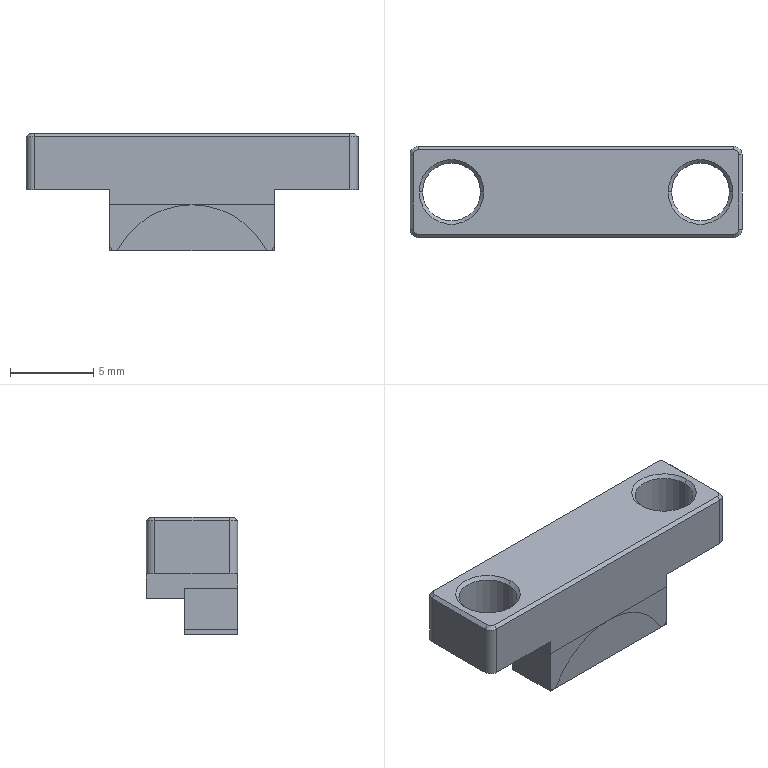Part | 2 solids | 42 faces | box 20 x 5.5 x 7.057 mm | volume 487.21 mm3 | plane 23 | cylinder 11 | cone 8 | commonest cylinder face diameters 1 x4 3.5 x4 0.6 x2 10 x1
STEP:
#1=CARTESIAN_POINT('',(4.95,-2.75,-4.3));
#2=VERTEX_POINT('',#1);
#3=CARTESIAN_POINT('',(-4.95,-2.75,-4.3));
#4=VERTEX_POINT('',#3);
#5=CARTESIAN_POINT('',(0.,-2.75,-4.3));
#6=DIRECTION('',(-1.,0.,0.));
#7=VECTOR('',#6,1000.);
#8=LINE('',#5,#7);
#9=EDGE_CURVE('',#2,#4,#8,.T.);
#10=ORIENTED_EDGE('',*,*,#9,.F.);
#11=CARTESIAN_POINT('',(4.95,0.45,-4.3));
#12=VERTEX_POINT('',#11);
#13=CARTESIAN_POINT('',(4.95,-1.15,-4.3));
#14=DIRECTION('',(0.,-1.,0.));
#15=VECTOR('',#14,1000.);
#16=LINE('',#13,#15);
#17=EDGE_CURVE('',#12,#2,#16,.T.);
#18=ORIENTED_EDGE('',*,*,#17,.F.);
#19=CARTESIAN_POINT('',(-4.95,0.45,-4.3));
#20=VERTEX_POINT('',#19);
#21=CARTESIAN_POINT('',(0.,0.45,-4.3));
#22=DIRECTION('',(1.,0.,0.));
#23=VECTOR('',#22,1000.);
#24=LINE('',#21,#23);
#25=EDGE_CURVE('',#20,#12,#24,.T.);
#26=ORIENTED_EDGE('',*,*,#25,.F.);
#27=CARTESIAN_POINT('',(-4.95,-1.15,-4.3));
#28=DIRECTION('',(0.,1.,0.));
#29=VECTOR('',#28,1000.);
#30=LINE('',#27,#29);
#31=EDGE_CURVE('',#4,#20,#30,.T.);
#32=ORIENTED_EDGE('',*,*,#31,.F.);
#33=EDGE_LOOP('',(#10,#18,#26,#32));
#34=FACE_BOUND('',#33,.T.);
#35=CARTESIAN_POINT('',(0.,-1.15,-4.3));
#36=DIRECTION('',(0.,0.,1.));
#37=DIRECTION('',(1.,0.,0.));
#38=AXIS2_PLACEMENT_3D('',#35,#36,#37);
#39=PLANE('',#38);
#40=ADVANCED_FACE('',(#34),#39,.T.);
#41=CARTESIAN_POINT('',(4.95,-2.75,-7.057));
#42=VERTEX_POINT('',#41);
#43=CARTESIAN_POINT('',(4.95,-2.75,-7.057));
#44=DIRECTION('',(0.,0.,1.));
#45=VECTOR('',#44,1000.);
#46=LINE('',#43,#45);
#47=EDGE_CURVE('',#42,#2,#46,.T.);
#48=ORIENTED_EDGE('',*,*,#47,.T.);
#49=ORIENTED_EDGE('',*,*,#9,.T.);
#50=CARTESIAN_POINT('',(-4.95,-2.75,-7.057));
#51=VERTEX_POINT('',#50);
#52=CARTESIAN_POINT('',(-4.95,-2.75,-7.057));
#53=DIRECTION('',(0.,0.,1.));
#54=VECTOR('',#53,1000.);
#55=LINE('',#52,#54);
#56=EDGE_CURVE('',#51,#4,#55,.T.);
#57=ORIENTED_EDGE('',*,*,#56,.F.);
#58=CARTESIAN_POINT('',(0.,-2.75,-7.057));
#59=DIRECTION('',(1.,0.,0.));
#60=VECTOR('',#59,1000.);
#61=LINE('',#58,#60);
#62=EDGE_CURVE('',#51,#42,#61,.T.);
#63=ORIENTED_EDGE('',*,*,#62,.T.);
#64=EDGE_LOOP('',(#48,#49,#57,#63));
#65=FACE_BOUND('',#64,.T.);
#66=CARTESIAN_POINT('',(0.,-2.75,-7.057));
#67=DIRECTION('',(0.,-1.,0.));
#68=DIRECTION('',(0.,0.,-1.));
#69=AXIS2_PLACEMENT_3D('',#66,#67,#68);
#70=PLANE('',#69);
#71=ADVANCED_FACE('',(#65),#70,.T.);
#72=ORIENTED_EDGE('',*,*,#56,.T.);
#73=ORIENTED_EDGE('',*,*,#31,.T.);
#74=CARTESIAN_POINT('',(-4.95,0.45,-7.057));
#75=VERTEX_POINT('',#74);
#76=CARTESIAN_POINT('',(-4.95,0.45,-7.057));
#77=DIRECTION('',(0.,0.,1.));
#78=VECTOR('',#77,1000.);
#79=LINE('',#76,#78);
#80=EDGE_CURVE('',#75,#20,#79,.T.);
#81=ORIENTED_EDGE('',*,*,#80,.F.);
#82=CARTESIAN_POINT('',(-4.95,-1.15,-7.057));
#83=DIRECTION('',(0.,-1.,0.));
#84=VECTOR('',#83,1000.);
#85=LINE('',#82,#84);
#86=EDGE_CURVE('',#75,#51,#85,.T.);
#87=ORIENTED_EDGE('',*,*,#86,.T.);
#88=EDGE_LOOP('',(#72,#73,#81,#87));
#89=FACE_BOUND('',#88,.T.);
#90=CARTESIAN_POINT('',(-4.95,-1.15,-7.057));
#91=DIRECTION('',(-1.,0.,0.));
#92=DIRECTION('',(0.,0.,1.));
#93=AXIS2_PLACEMENT_3D('',#90,#91,#92);
#94=PLANE('',#93);
#95=ADVANCED_FACE('',(#89),#94,.T.);
#96=ORIENTED_EDGE('',*,*,#80,.T.);
#97=ORIENTED_EDGE('',*,*,#25,.T.);
#98=CARTESIAN_POINT('',(4.95,0.45,-7.057));
#99=VERTEX_POINT('',#98);
#100=CARTESIAN_POINT('',(4.95,0.45,-7.057));
#101=DIRECTION('',(0.,0.,1.));
#102=VECTOR('',#101,1000.);
#103=LINE('',#100,#102);
#104=EDGE_CURVE('',#99,#12,#103,.T.);
#105=ORIENTED_EDGE('',*,*,#104,.F.);
#106=CARTESIAN_POINT('',(0.,0.45,-7.057));
#107=DIRECTION('',(-1.,0.,0.));
#108=VECTOR('',#107,1000.);
#109=LINE('',#106,#108);
#110=EDGE_CURVE('',#99,#75,#109,.T.);
#111=ORIENTED_EDGE('',*,*,#110,.T.);
#112=EDGE_LOOP('',(#96,#97,#105,#111));
#113=FACE_BOUND('',#112,.T.);
#114=CARTESIAN_POINT('',(0.,0.45,-7.057));
#115=DIRECTION('',(0.,1.,0.));
#116=DIRECTION('',(0.,0.,1.));
#117=AXIS2_PLACEMENT_3D('',#114,#115,#116);
#118=PLANE('',#117);
#119=ADVANCED_FACE('',(#113),#118,.T.);
#120=CARTESIAN_POINT('',(4.95,-1.15,-7.057));
#121=DIRECTION('',(0.,1.,0.));
#122=VECTOR('',#121,1000.);
#123=LINE('',#120,#122);
#124=EDGE_CURVE('',#42,#99,#123,.T.);
#125=ORIENTED_EDGE('',*,*,#124,.F.);
#126=ORIENTED_EDGE('',*,*,#62,.F.);
#127=ORIENTED_EDGE('',*,*,#86,.F.);
#128=ORIENTED_EDGE('',*,*,#110,.F.);
#129=EDGE_LOOP('',(#125,#126,#127,#128));
#130=FACE_BOUND('',#129,.T.);
#131=CARTESIAN_POINT('',(0.,-1.15,-7.057));
#132=DIRECTION('',(0.,0.,-1.));
#133=DIRECTION('',(-1.,0.,0.));
#134=AXIS2_PLACEMENT_3D('',#131,#132,#133);
#135=PLANE('',#134);
#136=ADVANCED_FACE('',(#130),#135,.T.);
#137=ORIENTED_EDGE('',*,*,#124,.T.);
#138=ORIENTED_EDGE('',*,*,#104,.T.);
#139=ORIENTED_EDGE('',*,*,#17,.T.);
#140=ORIENTED_EDGE('',*,*,#47,.F.);
#141=EDGE_LOOP('',(#137,#138,#139,#140));
#142=FACE_BOUND('',#141,.T.);
#143=CARTESIAN_POINT('',(4.95,-1.15,-7.057));
#144=DIRECTION('',(1.,0.,0.));
#145=DIRECTION('',(0.,0.,-1.));
#146=AXIS2_PLACEMENT_3D('',#143,#144,#145);
#147=PLANE('',#146);
#148=ADVANCED_FACE('',(#142),#147,.T.);
#149=CLOSED_SHELL('',(#40,#71,#95,#119,#136,#148));
#150=MANIFOLD_SOLID_BREP('',#149);
#151=CARTESIAN_POINT('',(9.5,2.75,-0.2));
#152=VERTEX_POINT('',#151);
#153=CARTESIAN_POINT('',(9.5,2.75,-3.4));
#154=VERTEX_POINT('',#153);
#155=CARTESIAN_POINT('',(9.5,2.75,-0.2));
#156=DIRECTION('',(-0.000000324,0.000000043,-1.));
#157=VECTOR('',#156,1000.);
#158=LINE('',#155,#157);
#159=EDGE_CURVE('',#152,#154,#158,.T.);
#160=ORIENTED_EDGE('',*,*,#159,.T.);
#161=CARTESIAN_POINT('',(4.95,2.75,-3.4));
#162=VERTEX_POINT('',#161);
#163=CARTESIAN_POINT('',(4.95,2.75,-3.4));
#164=DIRECTION('',(1.,0.,0.));
#165=VECTOR('',#164,1000.);
#166=LINE('',#163,#165);
#167=EDGE_CURVE('',#162,#154,#166,.T.);
#168=ORIENTED_EDGE('',*,*,#167,.F.);
#169=CARTESIAN_POINT('',(4.95,2.75,-4.9));
#170=VERTEX_POINT('',#169);
#171=CARTESIAN_POINT('',(4.95,2.75,-3.4));
#172=DIRECTION('',(0.,0.,-1.));
#173=VECTOR('',#172,1000.);
#174=LINE('',#171,#173);
#175=EDGE_CURVE('',#162,#170,#174,.T.);
#176=ORIENTED_EDGE('',*,*,#175,.T.);
#177=CARTESIAN_POINT('',(-4.95,2.75,-4.9));
#178=VERTEX_POINT('',#177);
#179=CARTESIAN_POINT('',(4.95,2.75,-4.9));
#180=DIRECTION('',(-1.,0.,0.));
#181=VECTOR('',#180,1000.);
#182=LINE('',#179,#181);
#183=EDGE_CURVE('',#170,#178,#182,.T.);
#184=ORIENTED_EDGE('',*,*,#183,.T.);
#185=CARTESIAN_POINT('',(-4.95,2.75,-3.4));
#186=VERTEX_POINT('',#185);
#187=CARTESIAN_POINT('',(-4.95,2.75,-4.9));
#188=DIRECTION('',(0.,0.,1.));
#189=VECTOR('',#188,1000.);
#190=LINE('',#187,#189);
#191=EDGE_CURVE('',#178,#186,#190,.T.);
#192=ORIENTED_EDGE('',*,*,#191,.T.);
#193=CARTESIAN_POINT('',(-9.5,2.75,-3.4));
#194=VERTEX_POINT('',#193);
#195=CARTESIAN_POINT('',(-9.5,2.75,-3.4));
#196=DIRECTION('',(1.,0.,0.));
#197=VECTOR('',#196,1000.);
#198=LINE('',#195,#197);
#199=EDGE_CURVE('',#194,#186,#198,.T.);
#200=ORIENTED_EDGE('',*,*,#199,.F.);
#201=CARTESIAN_POINT('',(-9.5,2.75,-0.2));
#202=VERTEX_POINT('',#201);
#203=CARTESIAN_POINT('',(-9.5,2.75,-3.4));
#204=DIRECTION('',(-0.000000324,-0.000000043,1.));
#205=VECTOR('',#204,1000.);
#206=LINE('',#203,#205);
#207=EDGE_CURVE('',#194,#202,#206,.T.);
#208=ORIENTED_EDGE('',*,*,#207,.T.);
#209=CARTESIAN_POINT('',(-9.5,2.75,-0.2));
#210=DIRECTION('',(1.,0.,0.));
#211=VECTOR('',#210,1000.);
#212=LINE('',#209,#211);
#213=EDGE_CURVE('',#202,#152,#212,.T.);
#214=ORIENTED_EDGE('',*,*,#213,.T.);
#215=EDGE_LOOP('',(#160,#168,#176,#184,#192,#200,#208,#214));
#216=FACE_BOUND('',#215,.T.);
#217=CARTESIAN_POINT('',(0.,2.75,-8.9));
#218=DIRECTION('',(0.,-1.,0.));
#219=DIRECTION('',(-1.,0.,0.));
#220=AXIS2_PLACEMENT_3D('',#217,#218,#219);
#221=PLANE('',#220);
#222=ADVANCED_FACE('',(#216),#221,.F.);
#223=CARTESIAN_POINT('',(-9.5,2.55,0.));
#224=VERTEX_POINT('',#223);
#225=CARTESIAN_POINT('',(-9.5,2.75,-0.2));
#226=DIRECTION('',(0.000000734,-0.7071,0.7071));
#227=VECTOR('',#226,1000.);
#228=LINE('',#225,#227);
#229=EDGE_CURVE('',#202,#224,#228,.T.);
#230=ORIENTED_EDGE('',*,*,#229,.T.);
#231=CARTESIAN_POINT('',(9.5,2.55,0.));
#232=VERTEX_POINT('',#231);
#233=CARTESIAN_POINT('',(-9.5,2.55,0.000000111));
#234=DIRECTION('',(1.,0.,0.));
#235=VECTOR('',#234,1000.);
#236=LINE('',#233,#235);
#237=EDGE_CURVE('',#224,#232,#236,.T.);
#238=ORIENTED_EDGE('',*,*,#237,.T.);
#239=CARTESIAN_POINT('',(9.5,2.75,-0.2));
#240=DIRECTION('',(-0.000000734,-0.7071,0.7071));
#241=VECTOR('',#240,1000.);
#242=LINE('',#239,#241);
#243=EDGE_CURVE('',#152,#232,#242,.T.);
#244=ORIENTED_EDGE('',*,*,#243,.F.);
#245=ORIENTED_EDGE('',*,*,#213,.F.);
#246=EDGE_LOOP('',(#230,#238,#244,#245));
#247=FACE_BOUND('',#246,.T.);
#248=CARTESIAN_POINT('',(0.,2.65,-0.1));
#249=DIRECTION('',(0.,0.7071,0.7071));
#250=DIRECTION('',(0.,0.7071,-0.7071));
#251=AXIS2_PLACEMENT_3D('',#248,#249,#250);
#252=PLANE('',#251);
#253=ADVANCED_FACE('',(#247),#252,.T.);
#254=ORIENTED_EDGE('',*,*,#243,.T.);
#255=CARTESIAN_POINT('',(9.8,2.25,0.));
#256=VERTEX_POINT('',#255);
#257=CARTESIAN_POINT('',(9.5,2.25,0.));
#258=DIRECTION('',(0.,0.,-1.));
#259=DIRECTION('',(0.,1.,0.));
#260=AXIS2_PLACEMENT_3D('',#257,#258,#259);
#261=CIRCLE('',#260,0.3);
#262=EDGE_CURVE('',#232,#256,#261,.T.);
#263=ORIENTED_EDGE('',*,*,#262,.T.);
#264=CARTESIAN_POINT('',(10.,2.25,-0.2));
#265=VERTEX_POINT('',#264);
#266=CARTESIAN_POINT('',(10.,2.25,-0.2));
#267=DIRECTION('',(-0.7071,-0.000000602,0.7071));
#268=VECTOR('',#267,1000.);
#269=LINE('',#266,#268);
#270=EDGE_CURVE('',#265,#256,#269,.T.);
#271=ORIENTED_EDGE('',*,*,#270,.F.);
#272=CARTESIAN_POINT('',(9.5,2.25,-0.2));
#273=DIRECTION('',(0.,0.,-1.));
#274=DIRECTION('',(0.,1.,0.));
#275=AXIS2_PLACEMENT_3D('',#272,#273,#274);
#276=CIRCLE('',#275,0.5);
#277=EDGE_CURVE('',#152,#265,#276,.T.);
#278=ORIENTED_EDGE('',*,*,#277,.F.);
#279=EDGE_LOOP('',(#254,#263,#271,#278));
#280=FACE_BOUND('',#279,.T.);
#281=CARTESIAN_POINT('',(9.5,2.25,-0.1));
#282=DIRECTION('',(0.,0.,-1.));
#283=DIRECTION('',(1.,0.,0.));
#284=AXIS2_PLACEMENT_3D('',#281,#282,#283);
#285=CONICAL_SURFACE('',#284,0.4,0.7854);
#286=ADVANCED_FACE('',(#280),#285,.T.);
#287=CARTESIAN_POINT('',(10.,2.25,-3.4));
#288=VERTEX_POINT('',#287);
#289=CARTESIAN_POINT('',(10.,2.25,-0.2));
#290=DIRECTION('',(0.000000046,-0.000000266,-1.));
#291=VECTOR('',#290,1000.);
#292=LINE('',#289,#291);
#293=EDGE_CURVE('',#265,#288,#292,.T.);
#294=ORIENTED_EDGE('',*,*,#293,.T.);
#295=CARTESIAN_POINT('',(9.5,2.25,-3.4));
#296=DIRECTION('',(0.,0.,-1.));
#297=DIRECTION('',(0.,1.,0.));
#298=AXIS2_PLACEMENT_3D('',#295,#296,#297);
#299=CIRCLE('',#298,0.5);
#300=EDGE_CURVE('',#154,#288,#299,.T.);
#301=ORIENTED_EDGE('',*,*,#300,.F.);
#302=ORIENTED_EDGE('',*,*,#159,.F.);
#303=ORIENTED_EDGE('',*,*,#277,.T.);
#304=EDGE_LOOP('',(#294,#301,#302,#303));
#305=FACE_BOUND('',#304,.T.);
#306=CARTESIAN_POINT('',(9.5,2.25,6.388));
#307=DIRECTION('',(0.,0.,-1.));
#308=DIRECTION('',(0.,-1.,0.));
#309=AXIS2_PLACEMENT_3D('',#306,#307,#308);
#310=CYLINDRICAL_SURFACE('',#309,0.5);
#311=ADVANCED_FACE('',(#305),#310,.T.);
#312=ORIENTED_EDGE('',*,*,#300,.T.);
#313=CARTESIAN_POINT('',(10.,-2.25,-3.4));
#314=VERTEX_POINT('',#313);
#315=CARTESIAN_POINT('',(10.,2.25,-3.4));
#316=DIRECTION('',(0.,-1.,0.));
#317=VECTOR('',#316,1000.);
#318=LINE('',#315,#317);
#319=EDGE_CURVE('',#288,#314,#318,.T.);
#320=ORIENTED_EDGE('',*,*,#319,.T.);
#321=CARTESIAN_POINT('',(9.5,-2.75,-3.4));
#322=VERTEX_POINT('',#321);
#323=CARTESIAN_POINT('',(9.5,-2.25,-3.4));
#324=DIRECTION('',(0.,0.,-1.));
#325=DIRECTION('',(1.,0.,0.));
#326=AXIS2_PLACEMENT_3D('',#323,#324,#325);
#327=CIRCLE('',#326,0.5);
#328=EDGE_CURVE('',#314,#322,#327,.T.);
#329=ORIENTED_EDGE('',*,*,#328,.T.);
#330=CARTESIAN_POINT('',(4.95,-2.75,-3.4));
#331=VERTEX_POINT('',#330);
#332=CARTESIAN_POINT('',(4.95,-2.75,-3.4));
#333=DIRECTION('',(1.,0.,0.));
#334=VECTOR('',#333,1000.);
#335=LINE('',#332,#334);
#336=EDGE_CURVE('',#331,#322,#335,.T.);
#337=ORIENTED_EDGE('',*,*,#336,.F.);
#338=CARTESIAN_POINT('',(4.95,2.75,-3.4));
#339=DIRECTION('',(0.,-1.,0.));
#340=VECTOR('',#339,1000.);
#341=LINE('',#338,#340);
#342=EDGE_CURVE('',#162,#331,#341,.T.);
#343=ORIENTED_EDGE('',*,*,#342,.F.);
#344=ORIENTED_EDGE('',*,*,#167,.T.);
#345=EDGE_LOOP('',(#312,#320,#329,#337,#343,#344));
#346=FACE_BOUND('',#345,.T.);
#347=CARTESIAN_POINT('',(5.75,0.,-3.4));
#348=VERTEX_POINT('',#347);
#349=CARTESIAN_POINT('',(9.25,0.,-3.4));
#350=VERTEX_POINT('',#349);
#351=CARTESIAN_POINT('',(7.5,0.,-3.4));
#352=DIRECTION('',(0.,0.,1.));
#353=DIRECTION('',(-1.,0.,0.));
#354=AXIS2_PLACEMENT_3D('',#351,#352,#353);
#355=CIRCLE('',#354,1.75);
#356=EDGE_CURVE('',#348,#350,#355,.T.);
#357=ORIENTED_EDGE('',*,*,#356,.T.);
#358=CARTESIAN_POINT('',(7.5,0.,-3.4));
#359=DIRECTION('',(0.,0.,1.));
#360=DIRECTION('',(1.,0.,0.));
#361=AXIS2_PLACEMENT_3D('',#358,#359,#360);
#362=CIRCLE('',#361,1.75);
#363=EDGE_CURVE('',#350,#348,#362,.T.);
#364=ORIENTED_EDGE('',*,*,#363,.T.);
#365=EDGE_LOOP('',(#357,#364));
#366=FACE_BOUND('',#365,.T.);
#367=CARTESIAN_POINT('',(4.95,2.75,-3.4));
#368=DIRECTION('',(0.,0.,-1.));
#369=DIRECTION('',(-1.,0.,0.));
#370=AXIS2_PLACEMENT_3D('',#367,#368,#369);
#371=PLANE('',#370);
#372=ADVANCED_FACE('',(#346,#366),#371,.T.);
#373=CARTESIAN_POINT('',(5.75,0.,-0.2));
#374=VERTEX_POINT('',#373);
#375=CARTESIAN_POINT('',(5.75,0.000000759,-0.2));
#376=DIRECTION('',(-0.00000006,-0.000000237,-1.));
#377=VECTOR('',#376,1000.);
#378=LINE('',#375,#377);
#379=EDGE_CURVE('',#374,#348,#378,.T.);
#380=ORIENTED_EDGE('',*,*,#379,.T.);
#381=ORIENTED_EDGE('',*,*,#363,.F.);
#382=CARTESIAN_POINT('',(9.25,0.,-0.2));
#383=VERTEX_POINT('',#382);
#384=CARTESIAN_POINT('',(9.25,-0.000000759,-0.2));
#385=DIRECTION('',(0.00000006,0.000000237,-1.));
#386=VECTOR('',#385,1000.);
#387=LINE('',#384,#386);
#388=EDGE_CURVE('',#383,#350,#387,.T.);
#389=ORIENTED_EDGE('',*,*,#388,.F.);
#390=CARTESIAN_POINT('',(7.5,0.,-0.2));
#391=DIRECTION('',(0.,0.,-1.));
#392=DIRECTION('',(-1.,0.,0.));
#393=AXIS2_PLACEMENT_3D('',#390,#391,#392);
#394=CIRCLE('',#393,1.75);
#395=EDGE_CURVE('',#374,#383,#394,.T.);
#396=ORIENTED_EDGE('',*,*,#395,.F.);
#397=EDGE_LOOP('',(#380,#381,#389,#396));
#398=FACE_BOUND('',#397,.T.);
#399=CARTESIAN_POINT('',(7.5,0.,0.));
#400=DIRECTION('',(0.,0.,1.));
#401=DIRECTION('',(-1.,0.,0.));
#402=AXIS2_PLACEMENT_3D('',#399,#400,#401);
#403=CYLINDRICAL_SURFACE('',#402,1.75);
#404=ADVANCED_FACE('',(#398),#403,.F.);
#405=CARTESIAN_POINT('',(5.55,0.,0.));
#406=VERTEX_POINT('',#405);
#407=CARTESIAN_POINT('',(5.55,0.000001127,-0.000000285));
#408=DIRECTION('',(0.7071,-0.000001303,-0.7071));
#409=VECTOR('',#408,1000.);
#410=LINE('',#407,#409);
#411=EDGE_CURVE('',#406,#374,#410,.T.);
#412=ORIENTED_EDGE('',*,*,#411,.T.);
#413=ORIENTED_EDGE('',*,*,#395,.T.);
#414=CARTESIAN_POINT('',(9.45,0.,0.));
#415=VERTEX_POINT('',#414);
#416=CARTESIAN_POINT('',(9.45,-0.000001127,-0.000000285));
#417=DIRECTION('',(-0.7071,0.000001303,-0.7071));
#418=VECTOR('',#417,1000.);
#419=LINE('',#416,#418);
#420=EDGE_CURVE('',#415,#383,#419,.T.);
#421=ORIENTED_EDGE('',*,*,#420,.F.);
#422=CARTESIAN_POINT('',(7.5,0.,0.));
#423=DIRECTION('',(0.,0.,-1.));
#424=DIRECTION('',(-1.,0.,0.));
#425=AXIS2_PLACEMENT_3D('',#422,#423,#424);
#426=CIRCLE('',#425,1.95);
#427=EDGE_CURVE('',#406,#415,#426,.T.);
#428=ORIENTED_EDGE('',*,*,#427,.F.);
#429=EDGE_LOOP('',(#412,#413,#421,#428));
#430=FACE_BOUND('',#429,.T.);
#431=CARTESIAN_POINT('',(7.5,0.,-0.1));
#432=DIRECTION('',(0.,0.,1.));
#433=DIRECTION('',(1.,0.,0.));
#434=AXIS2_PLACEMENT_3D('',#431,#432,#433);
#435=CONICAL_SURFACE('',#434,1.85,0.7854);
#436=ADVANCED_FACE('',(#430),#435,.F.);
#437=ORIENTED_EDGE('',*,*,#237,.F.);
#438=CARTESIAN_POINT('',(-9.8,2.25,0.000000117));
#439=VERTEX_POINT('',#438);
#440=CARTESIAN_POINT('',(-9.5,2.25,0.));
#441=DIRECTION('',(0.,0.,-1.));
#442=DIRECTION('',(-1.,0.,0.));
#443=AXIS2_PLACEMENT_3D('',#440,#441,#442);
#444=CIRCLE('',#443,0.3);
#445=EDGE_CURVE('',#439,#224,#444,.T.);
#446=ORIENTED_EDGE('',*,*,#445,.F.);
#447=CARTESIAN_POINT('',(-9.8,-2.25,0.));
#448=VERTEX_POINT('',#447);
#449=CARTESIAN_POINT('',(-9.8,-2.25,0.000000117));
#450=DIRECTION('',(0.,1.,0.));
#451=VECTOR('',#450,1000.);
#452=LINE('',#449,#451);
#453=EDGE_CURVE('',#448,#439,#452,.T.);
#454=ORIENTED_EDGE('',*,*,#453,.F.);
#455=CARTESIAN_POINT('',(-9.5,-2.55,0.000000111));
#456=VERTEX_POINT('',#455);
#457=CARTESIAN_POINT('',(-9.5,-2.25,0.));
#458=DIRECTION('',(0.,0.,-1.));
#459=DIRECTION('',(0.,-1.,0.));
#460=AXIS2_PLACEMENT_3D('',#457,#458,#459);
#461=CIRCLE('',#460,0.3);
#462=EDGE_CURVE('',#456,#448,#461,.T.);
#463=ORIENTED_EDGE('',*,*,#462,.F.);
#464=CARTESIAN_POINT('',(9.5,-2.55,0.));
#465=VERTEX_POINT('',#464);
#466=CARTESIAN_POINT('',(9.5,-2.55,0.000000111));
#467=DIRECTION('',(-1.,0.,0.));
#468=VECTOR('',#467,1000.);
#469=LINE('',#466,#468);
#470=EDGE_CURVE('',#465,#456,#469,.T.);
#471=ORIENTED_EDGE('',*,*,#470,.F.);
#472=CARTESIAN_POINT('',(9.8,-2.25,0.000000117));
#473=VERTEX_POINT('',#472);
#474=CARTESIAN_POINT('',(9.5,-2.25,0.));
#475=DIRECTION('',(0.,0.,-1.));
#476=DIRECTION('',(1.,0.,0.));
#477=AXIS2_PLACEMENT_3D('',#474,#475,#476);
#478=CIRCLE('',#477,0.3);
#479=EDGE_CURVE('',#473,#465,#478,.T.);
#480=ORIENTED_EDGE('',*,*,#479,.F.);
#481=CARTESIAN_POINT('',(9.8,2.25,0.000000117));
#482=DIRECTION('',(0.,-1.,0.));
#483=VECTOR('',#482,1000.);
#484=LINE('',#481,#483);
#485=EDGE_CURVE('',#256,#473,#484,.T.);
#486=ORIENTED_EDGE('',*,*,#485,.F.);
#487=ORIENTED_EDGE('',*,*,#262,.F.);
#488=EDGE_LOOP('',(#437,#446,#454,#463,#471,#480,#486,#487));
#489=FACE_BOUND('',#488,.T.);
#490=CARTESIAN_POINT('',(-9.45,0.,0.));
#491=VERTEX_POINT('',#490);
#492=CARTESIAN_POINT('',(-5.55,0.,0.));
#493=VERTEX_POINT('',#492);
#494=CARTESIAN_POINT('',(-7.5,0.,0.));
#495=DIRECTION('',(0.,0.,-1.));
#496=DIRECTION('',(-1.,0.,0.));
#497=AXIS2_PLACEMENT_3D('',#494,#495,#496);
#498=CIRCLE('',#497,1.95);
#499=EDGE_CURVE('',#491,#493,#498,.T.);
#500=ORIENTED_EDGE('',*,*,#499,.T.);
#501=CARTESIAN_POINT('',(-7.5,0.,0.));
#502=DIRECTION('',(0.,0.,-1.));
#503=DIRECTION('',(1.,0.,0.));
#504=AXIS2_PLACEMENT_3D('',#501,#502,#503);
#505=CIRCLE('',#504,1.95);
#506=EDGE_CURVE('',#493,#491,#505,.T.);
#507=ORIENTED_EDGE('',*,*,#506,.T.);
#508=EDGE_LOOP('',(#500,#507));
#509=FACE_BOUND('',#508,.T.);
#510=ORIENTED_EDGE('',*,*,#427,.T.);
#511=CARTESIAN_POINT('',(7.5,0.,0.));
#512=DIRECTION('',(0.,0.,-1.));
#513=DIRECTION('',(1.,0.,0.));
#514=AXIS2_PLACEMENT_3D('',#511,#512,#513);
#515=CIRCLE('',#514,1.95);
#516=EDGE_CURVE('',#415,#406,#515,.T.);
#517=ORIENTED_EDGE('',*,*,#516,.T.);
#518=EDGE_LOOP('',(#510,#517));
#519=FACE_BOUND('',#518,.T.);
#520=CARTESIAN_POINT('',(10.,2.75,0.));
#521=DIRECTION('',(0.,0.,1.));
#522=DIRECTION('',(1.,0.,0.));
#523=AXIS2_PLACEMENT_3D('',#520,#521,#522);
#524=PLANE('',#523);
#525=ADVANCED_FACE('',(#489,#509,#519),#524,.T.);
#526=ORIENTED_EDGE('',*,*,#420,.T.);
#527=CARTESIAN_POINT('',(7.5,0.,-0.2));
#528=DIRECTION('',(0.,0.,-1.));
#529=DIRECTION('',(1.,0.,0.));
#530=AXIS2_PLACEMENT_3D('',#527,#528,#529);
#531=CIRCLE('',#530,1.75);
#532=EDGE_CURVE('',#383,#374,#531,.T.);
#533=ORIENTED_EDGE('',*,*,#532,.T.);
#534=ORIENTED_EDGE('',*,*,#411,.F.);
#535=ORIENTED_EDGE('',*,*,#516,.F.);
#536=EDGE_LOOP('',(#526,#533,#534,#535));
#537=FACE_BOUND('',#536,.T.);
#538=CARTESIAN_POINT('',(7.5,0.,-0.1));
#539=DIRECTION('',(0.,0.,1.));
#540=DIRECTION('',(1.,0.,0.));
#541=AXIS2_PLACEMENT_3D('',#538,#539,#540);
#542=CONICAL_SURFACE('',#541,1.85,0.7854);
#543=ADVANCED_FACE('',(#537),#542,.F.);
#544=ORIENTED_EDGE('',*,*,#388,.T.);
#545=ORIENTED_EDGE('',*,*,#356,.F.);
#546=ORIENTED_EDGE('',*,*,#379,.F.);
#547=ORIENTED_EDGE('',*,*,#532,.F.);
#548=EDGE_LOOP('',(#544,#545,#546,#547));
#549=FACE_BOUND('',#548,.T.);
#550=CARTESIAN_POINT('',(7.5,0.,0.));
#551=DIRECTION('',(0.,0.,1.));
#552=DIRECTION('',(-1.,0.,0.));
#553=AXIS2_PLACEMENT_3D('',#550,#551,#552);
#554=CYLINDRICAL_SURFACE('',#553,1.75);
#555=ADVANCED_FACE('',(#549),#554,.F.);
#556=CARTESIAN_POINT('',(-5.75,0.,-0.2));
#557=VERTEX_POINT('',#556);
#558=CARTESIAN_POINT('',(-5.55,-0.000001127,-0.000000285));
#559=DIRECTION('',(-0.7071,0.000001303,-0.7071));
#560=VECTOR('',#559,1000.);
#561=LINE('',#558,#560);
#562=EDGE_CURVE('',#493,#557,#561,.T.);
#563=ORIENTED_EDGE('',*,*,#562,.T.);
#564=CARTESIAN_POINT('',(-9.25,0.,-0.2));
#565=VERTEX_POINT('',#564);
#566=CARTESIAN_POINT('',(-7.5,0.,-0.2));
#567=DIRECTION('',(0.,0.,-1.));
#568=DIRECTION('',(1.,0.,0.));
#569=AXIS2_PLACEMENT_3D('',#566,#567,#568);
#570=CIRCLE('',#569,1.75);
#571=EDGE_CURVE('',#557,#565,#570,.T.);
#572=ORIENTED_EDGE('',*,*,#571,.T.);
#573=CARTESIAN_POINT('',(-9.45,0.000001127,-0.000000285));
#574=DIRECTION('',(0.7071,-0.000001303,-0.7071));
#575=VECTOR('',#574,1000.);
#576=LINE('',#573,#575);
#577=EDGE_CURVE('',#491,#565,#576,.T.);
#578=ORIENTED_EDGE('',*,*,#577,.F.);
#579=ORIENTED_EDGE('',*,*,#506,.F.);
#580=EDGE_LOOP('',(#563,#572,#578,#579));
#581=FACE_BOUND('',#580,.T.);
#582=CARTESIAN_POINT('',(-7.5,0.,-0.1));
#583=DIRECTION('',(0.,0.,1.));
#584=DIRECTION('',(1.,0.,0.));
#585=AXIS2_PLACEMENT_3D('',#582,#583,#584);
#586=CONICAL_SURFACE('',#585,1.85,0.7854);
#587=ADVANCED_FACE('',(#581),#586,.F.);
#588=ORIENTED_EDGE('',*,*,#577,.T.);
#589=CARTESIAN_POINT('',(-7.5,0.,-0.2));
#590=DIRECTION('',(0.,0.,-1.));
#591=DIRECTION('',(-1.,0.,0.));
#592=AXIS2_PLACEMENT_3D('',#589,#590,#591);
#593=CIRCLE('',#592,1.75);
#594=EDGE_CURVE('',#565,#557,#593,.T.);
#595=ORIENTED_EDGE('',*,*,#594,.T.);
#596=ORIENTED_EDGE('',*,*,#562,.F.);
#597=ORIENTED_EDGE('',*,*,#499,.F.);
#598=EDGE_LOOP('',(#588,#595,#596,#597));
#599=FACE_BOUND('',#598,.T.);
#600=CARTESIAN_POINT('',(-7.5,0.,-0.1));
#601=DIRECTION('',(0.,0.,1.));
#602=DIRECTION('',(1.,0.,0.));
#603=AXIS2_PLACEMENT_3D('',#600,#601,#602);
#604=CONICAL_SURFACE('',#603,1.85,0.7854);
#605=ADVANCED_FACE('',(#599),#604,.F.);
#606=CARTESIAN_POINT('',(-9.25,0.,-3.4));
#607=VERTEX_POINT('',#606);
#608=CARTESIAN_POINT('',(-9.25,0.000000759,-0.2));
#609=DIRECTION('',(-0.00000006,-0.000000237,-1.));
#610=VECTOR('',#609,1000.);
#611=LINE('',#608,#610);
#612=EDGE_CURVE('',#565,#607,#611,.T.);
#613=ORIENTED_EDGE('',*,*,#612,.T.);
#614=CARTESIAN_POINT('',(-5.75,0.,-3.4));
#615=VERTEX_POINT('',#614);
#616=CARTESIAN_POINT('',(-7.5,0.,-3.4));
#617=DIRECTION('',(0.,0.,1.));
#618=DIRECTION('',(1.,0.,0.));
#619=AXIS2_PLACEMENT_3D('',#616,#617,#618);
#620=CIRCLE('',#619,1.75);
#621=EDGE_CURVE('',#615,#607,#620,.T.);
#622=ORIENTED_EDGE('',*,*,#621,.F.);
#623=CARTESIAN_POINT('',(-5.75,-0.000000759,-0.2));
#624=DIRECTION('',(0.00000006,0.000000237,-1.));
#625=VECTOR('',#624,1000.);
#626=LINE('',#623,#625);
#627=EDGE_CURVE('',#557,#615,#626,.T.);
#628=ORIENTED_EDGE('',*,*,#627,.F.);
#629=ORIENTED_EDGE('',*,*,#594,.F.);
#630=EDGE_LOOP('',(#613,#622,#628,#629));
#631=FACE_BOUND('',#630,.T.);
#632=CARTESIAN_POINT('',(-7.5,0.,0.));
#633=DIRECTION('',(0.,0.,1.));
#634=DIRECTION('',(-1.,0.,0.));
#635=AXIS2_PLACEMENT_3D('',#632,#633,#634);
#636=CYLINDRICAL_SURFACE('',#635,1.75);
#637=ADVANCED_FACE('',(#631),#636,.F.);
#638=ORIENTED_EDGE('',*,*,#627,.T.);
#639=CARTESIAN_POINT('',(-7.5,0.,-3.4));
#640=DIRECTION('',(0.,0.,1.));
#641=DIRECTION('',(-1.,0.,0.));
#642=AXIS2_PLACEMENT_3D('',#639,#640,#641);
#643=CIRCLE('',#642,1.75);
#644=EDGE_CURVE('',#607,#615,#643,.T.);
#645=ORIENTED_EDGE('',*,*,#644,.F.);
#646=ORIENTED_EDGE('',*,*,#612,.F.);
#647=ORIENTED_EDGE('',*,*,#571,.F.);
#648=EDGE_LOOP('',(#638,#645,#646,#647));
#649=FACE_BOUND('',#648,.T.);
#650=CARTESIAN_POINT('',(-7.5,0.,0.));
#651=DIRECTION('',(0.,0.,1.));
#652=DIRECTION('',(-1.,0.,0.));
#653=AXIS2_PLACEMENT_3D('',#650,#651,#652);
#654=CYLINDRICAL_SURFACE('',#653,1.75);
#655=ADVANCED_FACE('',(#649),#654,.F.);
#656=CARTESIAN_POINT('',(-4.95,-2.75,-3.4));
#657=VERTEX_POINT('',#656);
#658=CARTESIAN_POINT('',(-4.95,2.75,-3.4));
#659=DIRECTION('',(0.,-1.,0.));
#660=VECTOR('',#659,1000.);
#661=LINE('',#658,#660);
#662=EDGE_CURVE('',#186,#657,#661,.T.);
#663=ORIENTED_EDGE('',*,*,#662,.T.);
#664=CARTESIAN_POINT('',(-9.5,-2.75,-3.4));
#665=VERTEX_POINT('',#664);
#666=CARTESIAN_POINT('',(-9.5,-2.75,-3.4));
#667=DIRECTION('',(1.,0.,0.));
#668=VECTOR('',#667,1000.);
#669=LINE('',#666,#668);
#670=EDGE_CURVE('',#665,#657,#669,.T.);
#671=ORIENTED_EDGE('',*,*,#670,.F.);
#672=CARTESIAN_POINT('',(-10.,-2.25,-3.4));
#673=VERTEX_POINT('',#672);
#674=CARTESIAN_POINT('',(-9.5,-2.25,-3.4));
#675=DIRECTION('',(0.,0.,-1.));
#676=DIRECTION('',(0.,-1.,0.));
#677=AXIS2_PLACEMENT_3D('',#674,#675,#676);
#678=CIRCLE('',#677,0.5);
#679=EDGE_CURVE('',#665,#673,#678,.T.);
#680=ORIENTED_EDGE('',*,*,#679,.T.);
#681=CARTESIAN_POINT('',(-10.,2.25,-3.4));
#682=VERTEX_POINT('',#681);
#683=CARTESIAN_POINT('',(-10.,2.25,-3.4));
#684=DIRECTION('',(0.,-1.,0.));
#685=VECTOR('',#684,1000.);
#686=LINE('',#683,#685);
#687=EDGE_CURVE('',#682,#673,#686,.T.);
#688=ORIENTED_EDGE('',*,*,#687,.F.);
#689=CARTESIAN_POINT('',(-9.5,2.25,-3.4));
#690=DIRECTION('',(0.,0.,-1.));
#691=DIRECTION('',(-1.,0.,0.));
#692=AXIS2_PLACEMENT_3D('',#689,#690,#691);
#693=CIRCLE('',#692,0.5);
#694=EDGE_CURVE('',#682,#194,#693,.T.);
#695=ORIENTED_EDGE('',*,*,#694,.T.);
#696=ORIENTED_EDGE('',*,*,#199,.T.);
#697=EDGE_LOOP('',(#663,#671,#680,#688,#695,#696));
#698=FACE_BOUND('',#697,.T.);
#699=ORIENTED_EDGE('',*,*,#644,.T.);
#700=ORIENTED_EDGE('',*,*,#621,.T.);
#701=EDGE_LOOP('',(#699,#700));
#702=FACE_BOUND('',#701,.T.);
#703=CARTESIAN_POINT('',(-10.,2.75,-3.4));
#704=DIRECTION('',(0.,0.,-1.));
#705=DIRECTION('',(-1.,0.,0.));
#706=AXIS2_PLACEMENT_3D('',#703,#704,#705);
#707=PLANE('',#706);
#708=ADVANCED_FACE('',(#698,#702),#707,.T.);
#709=ORIENTED_EDGE('',*,*,#207,.F.);
#710=ORIENTED_EDGE('',*,*,#694,.F.);
#711=CARTESIAN_POINT('',(-10.,2.25,-0.2));
#712=VERTEX_POINT('',#711);
#713=CARTESIAN_POINT('',(-10.,2.25,-3.4));
#714=DIRECTION('',(0.000000046,0.000000266,1.));
#715=VECTOR('',#714,1000.);
#716=LINE('',#713,#715);
#717=EDGE_CURVE('',#682,#712,#716,.T.);
#718=ORIENTED_EDGE('',*,*,#717,.T.);
#719=CARTESIAN_POINT('',(-9.5,2.25,-0.2));
#720=DIRECTION('',(0.,0.,-1.));
#721=DIRECTION('',(-1.,0.,0.));
#722=AXIS2_PLACEMENT_3D('',#719,#720,#721);
#723=CIRCLE('',#722,0.5);
#724=EDGE_CURVE('',#712,#202,#723,.T.);
#725=ORIENTED_EDGE('',*,*,#724,.T.);
#726=EDGE_LOOP('',(#709,#710,#718,#725));
#727=FACE_BOUND('',#726,.T.);
#728=CARTESIAN_POINT('',(-9.5,2.25,-11.288));
#729=DIRECTION('',(0.,0.,1.));
#730=DIRECTION('',(0.,-1.,0.));
#731=AXIS2_PLACEMENT_3D('',#728,#729,#730);
#732=CYLINDRICAL_SURFACE('',#731,0.5);
#733=ADVANCED_FACE('',(#727),#732,.T.);
#734=CARTESIAN_POINT('',(-10.,2.25,-0.2));
#735=DIRECTION('',(0.7071,-0.000000602,0.7071));
#736=VECTOR('',#735,1000.);
#737=LINE('',#734,#736);
#738=EDGE_CURVE('',#712,#439,#737,.T.);
#739=ORIENTED_EDGE('',*,*,#738,.T.);
#740=ORIENTED_EDGE('',*,*,#445,.T.);
#741=ORIENTED_EDGE('',*,*,#229,.F.);
#742=ORIENTED_EDGE('',*,*,#724,.F.);
#743=EDGE_LOOP('',(#739,#740,#741,#742));
#744=FACE_BOUND('',#743,.T.);
#745=CARTESIAN_POINT('',(-9.5,2.25,-0.1));
#746=DIRECTION('',(0.,0.,-1.));
#747=DIRECTION('',(1.,0.,0.));
#748=AXIS2_PLACEMENT_3D('',#745,#746,#747);
#749=CONICAL_SURFACE('',#748,0.4,0.7854);
#750=ADVANCED_FACE('',(#744),#749,.T.);
#751=CARTESIAN_POINT('',(-10.,-2.25,-0.2));
#752=VERTEX_POINT('',#751);
#753=CARTESIAN_POINT('',(-10.,-2.25,-0.2));
#754=DIRECTION('',(0.7071,0.000000602,0.7071));
#755=VECTOR('',#754,1000.);
#756=LINE('',#753,#755);
#757=EDGE_CURVE('',#752,#448,#756,.T.);
#758=ORIENTED_EDGE('',*,*,#757,.T.);
#759=ORIENTED_EDGE('',*,*,#453,.T.);
#760=ORIENTED_EDGE('',*,*,#738,.F.);
#761=CARTESIAN_POINT('',(-10.,-2.25,-0.2));
#762=DIRECTION('',(0.,1.,0.));
#763=VECTOR('',#762,1000.);
#764=LINE('',#761,#763);
#765=EDGE_CURVE('',#752,#712,#764,.T.);
#766=ORIENTED_EDGE('',*,*,#765,.F.);
#767=EDGE_LOOP('',(#758,#759,#760,#766));
#768=FACE_BOUND('',#767,.T.);
#769=CARTESIAN_POINT('',(-9.9,0.,-0.1));
#770=DIRECTION('',(-0.7071,0.,0.7071));
#771=DIRECTION('',(-0.7071,0.,-0.7071));
#772=AXIS2_PLACEMENT_3D('',#769,#770,#771);
#773=PLANE('',#772);
#774=ADVANCED_FACE('',(#768),#773,.T.);
#775=ORIENTED_EDGE('',*,*,#717,.F.);
#776=ORIENTED_EDGE('',*,*,#687,.T.);
#777=CARTESIAN_POINT('',(-10.,-2.25,-0.2));
#778=DIRECTION('',(-0.000000046,0.000000266,-1.));
#779=VECTOR('',#778,1000.);
#780=LINE('',#777,#779);
#781=EDGE_CURVE('',#752,#673,#780,.T.);
#782=ORIENTED_EDGE('',*,*,#781,.F.);
#783=ORIENTED_EDGE('',*,*,#765,.T.);
#784=EDGE_LOOP('',(#775,#776,#782,#783));
#785=FACE_BOUND('',#784,.T.);
#786=CARTESIAN_POINT('',(-10.,2.75,0.));
#787=DIRECTION('',(-1.,0.,0.));
#788=DIRECTION('',(0.,0.,1.));
#789=AXIS2_PLACEMENT_3D('',#786,#787,#788);
#790=PLANE('',#789);
#791=ADVANCED_FACE('',(#785),#790,.T.);
#792=ORIENTED_EDGE('',*,*,#781,.T.);
#793=ORIENTED_EDGE('',*,*,#679,.F.);
#794=CARTESIAN_POINT('',(-9.5,-2.75,-0.2));
#795=VERTEX_POINT('',#794);
#796=CARTESIAN_POINT('',(-9.5,-2.75,-0.2));
#797=DIRECTION('',(0.000000324,-0.000000043,-1.));
#798=VECTOR('',#797,1000.);
#799=LINE('',#796,#798);
#800=EDGE_CURVE('',#795,#665,#799,.T.);
#801=ORIENTED_EDGE('',*,*,#800,.F.);
#802=CARTESIAN_POINT('',(-9.5,-2.25,-0.2));
#803=DIRECTION('',(0.,0.,-1.));
#804=DIRECTION('',(0.,-1.,0.));
#805=AXIS2_PLACEMENT_3D('',#802,#803,#804);
#806=CIRCLE('',#805,0.5);
#807=EDGE_CURVE('',#795,#752,#806,.T.);
#808=ORIENTED_EDGE('',*,*,#807,.T.);
#809=EDGE_LOOP('',(#792,#793,#801,#808));
#810=FACE_BOUND('',#809,.T.);
#811=CARTESIAN_POINT('',(-9.5,-2.25,6.388));
#812=DIRECTION('',(0.,0.,-1.));
#813=DIRECTION('',(0.,1.,0.));
#814=AXIS2_PLACEMENT_3D('',#811,#812,#813);
#815=CYLINDRICAL_SURFACE('',#814,0.5);
#816=ADVANCED_FACE('',(#810),#815,.T.);
#817=CARTESIAN_POINT('',(-9.5,-2.75,-0.2));
#818=DIRECTION('',(0.000000734,0.7071,0.7071));
#819=VECTOR('',#818,1000.);
#820=LINE('',#817,#819);
#821=EDGE_CURVE('',#795,#456,#820,.T.);
#822=ORIENTED_EDGE('',*,*,#821,.T.);
#823=ORIENTED_EDGE('',*,*,#462,.T.);
#824=ORIENTED_EDGE('',*,*,#757,.F.);
#825=ORIENTED_EDGE('',*,*,#807,.F.);
#826=EDGE_LOOP('',(#822,#823,#824,#825));
#827=FACE_BOUND('',#826,.T.);
#828=CARTESIAN_POINT('',(-9.5,-2.25,-0.1));
#829=DIRECTION('',(0.,0.,-1.));
#830=DIRECTION('',(1.,0.,0.));
#831=AXIS2_PLACEMENT_3D('',#828,#829,#830);
#832=CONICAL_SURFACE('',#831,0.4,0.7854);
#833=ADVANCED_FACE('',(#827),#832,.T.);
#834=CARTESIAN_POINT('',(9.5,-2.75,-0.2));
#835=VERTEX_POINT('',#834);
#836=CARTESIAN_POINT('',(9.5,-2.75,-0.2));
#837=DIRECTION('',(-0.000000734,0.7071,0.7071));
#838=VECTOR('',#837,1000.);
#839=LINE('',#836,#838);
#840=EDGE_CURVE('',#835,#465,#839,.T.);
#841=ORIENTED_EDGE('',*,*,#840,.T.);
#842=ORIENTED_EDGE('',*,*,#470,.T.);
#843=ORIENTED_EDGE('',*,*,#821,.F.);
#844=CARTESIAN_POINT('',(9.5,-2.75,-0.2));
#845=DIRECTION('',(-1.,0.,0.));
#846=VECTOR('',#845,1000.);
#847=LINE('',#844,#846);
#848=EDGE_CURVE('',#835,#795,#847,.T.);
#849=ORIENTED_EDGE('',*,*,#848,.F.);
#850=EDGE_LOOP('',(#841,#842,#843,#849));
#851=FACE_BOUND('',#850,.T.);
#852=CARTESIAN_POINT('',(0.,-2.65,-0.1));
#853=DIRECTION('',(0.,-0.7071,0.7071));
#854=DIRECTION('',(0.,-0.7071,-0.7071));
#855=AXIS2_PLACEMENT_3D('',#852,#853,#854);
#856=PLANE('',#855);
#857=ADVANCED_FACE('',(#851),#856,.T.);
#858=CARTESIAN_POINT('',(-4.387,-2.75,-6.901));
#859=VERTEX_POINT('',#858);
#860=CARTESIAN_POINT('',(4.387,-2.75,-6.901));
#861=VERTEX_POINT('',#860);
#862=CARTESIAN_POINT('',(0.,-2.75,-9.3));
#863=DIRECTION('',(0.,1.,0.));
#864=DIRECTION('',(-0.8774,0.,0.4798));
#865=AXIS2_PLACEMENT_3D('',#862,#863,#864);
#866=CIRCLE('',#865,5.);
#867=EDGE_CURVE('',#859,#861,#866,.T.);
#868=ORIENTED_EDGE('',*,*,#867,.T.);
#869=CARTESIAN_POINT('',(4.95,-2.75,-6.757));
#870=VERTEX_POINT('',#869);
#871=CARTESIAN_POINT('',(4.65,-2.75,-6.757));
#872=DIRECTION('',(0.,-1.,0.));
#873=DIRECTION('',(-0.8774,0.,-0.4798));
#874=AXIS2_PLACEMENT_3D('',#871,#872,#873);
#875=CIRCLE('',#874,0.3);
#876=EDGE_CURVE('',#861,#870,#875,.T.);
#877=ORIENTED_EDGE('',*,*,#876,.T.);
#878=CARTESIAN_POINT('',(4.95,-2.75,-6.757));
#879=DIRECTION('',(0.,0.,1.));
#880=VECTOR('',#879,1000.);
#881=LINE('',#878,#880);
#882=EDGE_CURVE('',#870,#331,#881,.T.);
#883=ORIENTED_EDGE('',*,*,#882,.T.);
#884=ORIENTED_EDGE('',*,*,#336,.T.);
#885=CARTESIAN_POINT('',(9.5,-2.75,-3.4));
#886=DIRECTION('',(0.000000324,0.000000043,1.));
#887=VECTOR('',#886,1000.);
#888=LINE('',#885,#887);
#889=EDGE_CURVE('',#322,#835,#888,.T.);
#890=ORIENTED_EDGE('',*,*,#889,.T.);
#891=ORIENTED_EDGE('',*,*,#848,.T.);
#892=ORIENTED_EDGE('',*,*,#800,.T.);
#893=ORIENTED_EDGE('',*,*,#670,.T.);
#894=CARTESIAN_POINT('',(-4.95,-2.75,-6.757));
#895=VERTEX_POINT('',#894);
#896=CARTESIAN_POINT('',(-4.95,-2.75,-3.4));
#897=DIRECTION('',(0.,0.,-1.));
#898=VECTOR('',#897,1000.);
#899=LINE('',#896,#898);
#900=EDGE_CURVE('',#657,#895,#899,.T.);
#901=ORIENTED_EDGE('',*,*,#900,.T.);
#902=CARTESIAN_POINT('',(-4.65,-2.75,-6.757));
#903=DIRECTION('',(0.,-1.,0.));
#904=DIRECTION('',(-1.,0.,0.));
#905=AXIS2_PLACEMENT_3D('',#902,#903,#904);
#906=CIRCLE('',#905,0.3);
#907=EDGE_CURVE('',#895,#859,#906,.T.);
#908=ORIENTED_EDGE('',*,*,#907,.T.);
#909=EDGE_LOOP('',(#868,#877,#883,#884,#890,#891,#892,#893,#901,#908));
#910=FACE_BOUND('',#909,.T.);
#911=CARTESIAN_POINT('',(0.,-2.75,-8.9));
#912=DIRECTION('',(0.,-1.,0.));
#913=DIRECTION('',(-1.,0.,0.));
#914=AXIS2_PLACEMENT_3D('',#911,#912,#913);
#915=PLANE('',#914);
#916=ADVANCED_FACE('',(#910),#915,.T.);
#917=CARTESIAN_POINT('',(-4.387,0.45,-6.901));
#918=VERTEX_POINT('',#917);
#919=CARTESIAN_POINT('',(-4.387,-2.75,-6.901));
#920=DIRECTION('',(0.,1.,0.));
#921=VECTOR('',#920,1000.);
#922=LINE('',#919,#921);
#923=EDGE_CURVE('',#859,#918,#922,.T.);
#924=ORIENTED_EDGE('',*,*,#923,.F.);
#925=ORIENTED_EDGE('',*,*,#907,.F.);
#926=CARTESIAN_POINT('',(-4.95,0.45,-6.757));
#927=VERTEX_POINT('',#926);
#928=CARTESIAN_POINT('',(-4.95,-2.75,-6.757));
#929=DIRECTION('',(0.,1.,0.));
#930=VECTOR('',#929,1000.);
#931=LINE('',#928,#930);
#932=EDGE_CURVE('',#895,#927,#931,.T.);
#933=ORIENTED_EDGE('',*,*,#932,.T.);
#934=CARTESIAN_POINT('',(-4.65,0.45,-6.757));
#935=DIRECTION('',(0.,1.,0.));
#936=DIRECTION('',(0.8774,0.,-0.4798));
#937=AXIS2_PLACEMENT_3D('',#934,#935,#936);
#938=CIRCLE('',#937,0.3);
#939=EDGE_CURVE('',#918,#927,#938,.T.);
#940=ORIENTED_EDGE('',*,*,#939,.F.);
#941=EDGE_LOOP('',(#924,#925,#933,#940));
#942=FACE_BOUND('',#941,.T.);
#943=CARTESIAN_POINT('',(-4.65,-9.92,-6.757));
#944=DIRECTION('',(0.,1.,0.));
#945=DIRECTION('',(-0.8774,0.,0.4798));
#946=AXIS2_PLACEMENT_3D('',#943,#944,#945);
#947=CYLINDRICAL_SURFACE('',#946,0.3);
#948=ADVANCED_FACE('',(#942),#947,.T.);
#949=CARTESIAN_POINT('',(-4.95,0.45,-4.9));
#950=VERTEX_POINT('',#949);
#951=CARTESIAN_POINT('',(-4.95,0.45,-4.9));
#952=DIRECTION('',(0.,0.,-1.));
#953=VECTOR('',#952,1000.);
#954=LINE('',#951,#953);
#955=EDGE_CURVE('',#950,#927,#954,.T.);
#956=ORIENTED_EDGE('',*,*,#955,.F.);
#957=CARTESIAN_POINT('',(-2.375,0.45,-4.9));
#958=VERTEX_POINT('',#957);
#959=CARTESIAN_POINT('',(-2.375,0.45,-4.9));
#960=DIRECTION('',(-1.,0.,0.));
#961=VECTOR('',#960,1000.);
#962=LINE('',#959,#961);
#963=EDGE_CURVE('',#958,#950,#962,.T.);
#964=ORIENTED_EDGE('',*,*,#963,.F.);
#965=CARTESIAN_POINT('',(0.,0.45,-9.3));
#966=DIRECTION('',(0.,1.,0.));
#967=DIRECTION('',(-0.8774,0.,0.4798));
#968=AXIS2_PLACEMENT_3D('',#965,#966,#967);
#969=CIRCLE('',#968,5.);
#970=EDGE_CURVE('',#918,#958,#969,.T.);
#971=ORIENTED_EDGE('',*,*,#970,.F.);
#972=ORIENTED_EDGE('',*,*,#939,.T.);
#973=EDGE_LOOP('',(#956,#964,#971,#972));
#974=FACE_BOUND('',#973,.T.);
#975=CARTESIAN_POINT('',(0.,0.45,-8.9));
#976=DIRECTION('',(0.,1.,0.));
#977=DIRECTION('',(-1.,0.,0.));
#978=AXIS2_PLACEMENT_3D('',#975,#976,#977);
#979=PLANE('',#978);
#980=ADVANCED_FACE('',(#974),#979,.T.);
#981=CARTESIAN_POINT('',(2.375,0.45,-4.9));
#982=VERTEX_POINT('',#981);
#983=CARTESIAN_POINT('',(4.387,0.45,-6.901));
#984=VERTEX_POINT('',#983);
#985=CARTESIAN_POINT('',(0.,0.45,-9.3));
#986=DIRECTION('',(0.,1.,0.));
#987=DIRECTION('',(0.475,0.,0.88));
#988=AXIS2_PLACEMENT_3D('',#985,#986,#987);
#989=CIRCLE('',#988,5.);
#990=EDGE_CURVE('',#982,#984,#989,.T.);
#991=ORIENTED_EDGE('',*,*,#990,.F.);
#992=CARTESIAN_POINT('',(4.95,0.45,-4.9));
#993=VERTEX_POINT('',#992);
#994=CARTESIAN_POINT('',(4.95,0.45,-4.9));
#995=DIRECTION('',(-1.,0.,0.));
#996=VECTOR('',#995,1000.);
#997=LINE('',#994,#996);
#998=EDGE_CURVE('',#993,#982,#997,.T.);
#999=ORIENTED_EDGE('',*,*,#998,.F.);
#1000=CARTESIAN_POINT('',(4.95,0.45,-6.757));
#1001=VERTEX_POINT('',#1000);
#1002=CARTESIAN_POINT('',(4.95,0.45,-6.757));
#1003=DIRECTION('',(0.,0.,1.));
#1004=VECTOR('',#1003,1000.);
#1005=LINE('',#1002,#1004);
#1006=EDGE_CURVE('',#1001,#993,#1005,.T.);
#1007=ORIENTED_EDGE('',*,*,#1006,.F.);
#1008=CARTESIAN_POINT('',(4.65,0.45,-6.757));
#1009=DIRECTION('',(0.,1.,0.));
#1010=DIRECTION('',(1.,0.,0.));
#1011=AXIS2_PLACEMENT_3D('',#1008,#1009,#1010);
#1012=CIRCLE('',#1011,0.3);
#1013=EDGE_CURVE('',#1001,#984,#1012,.T.);
#1014=ORIENTED_EDGE('',*,*,#1013,.T.);
#1015=EDGE_LOOP('',(#991,#999,#1007,#1014));
#1016=FACE_BOUND('',#1015,.T.);
#1017=CARTESIAN_POINT('',(0.,0.45,-8.9));
#1018=DIRECTION('',(0.,1.,0.));
#1019=DIRECTION('',(-1.,0.,0.));
#1020=AXIS2_PLACEMENT_3D('',#1017,#1018,#1019);
#1021=PLANE('',#1020);
#1022=ADVANCED_FACE('',(#1016),#1021,.T.);
#1023=ORIENTED_EDGE('',*,*,#970,.T.);
#1024=CARTESIAN_POINT('',(0.,0.45,-9.3));
#1025=DIRECTION('',(0.,-1.,0.));
#1026=DIRECTION('',(0.475,0.,0.88));
#1027=AXIS2_PLACEMENT_3D('',#1024,#1025,#1026);
#1028=CIRCLE('',#1027,5.);
#1029=EDGE_CURVE('',#982,#958,#1028,.T.);
#1030=ORIENTED_EDGE('',*,*,#1029,.F.);
#1031=ORIENTED_EDGE('',*,*,#990,.T.);
#1032=CARTESIAN_POINT('',(4.387,-2.75,-6.901));
#1033=DIRECTION('',(0.,1.,0.));
#1034=VECTOR('',#1033,1000.);
#1035=LINE('',#1032,#1034);
#1036=EDGE_CURVE('',#861,#984,#1035,.T.);
#1037=ORIENTED_EDGE('',*,*,#1036,.F.);
#1038=ORIENTED_EDGE('',*,*,#867,.F.);
#1039=ORIENTED_EDGE('',*,*,#923,.T.);
#1040=EDGE_LOOP('',(#1023,#1030,#1031,#1037,#1038,#1039));
#1041=FACE_BOUND('',#1040,.T.);
#1042=CARTESIAN_POINT('',(0.,-2.75,-9.3));
#1043=DIRECTION('',(0.,-1.,0.));
#1044=DIRECTION('',(-1.,0.,0.));
#1045=AXIS2_PLACEMENT_3D('',#1042,#1043,#1044);
#1046=CYLINDRICAL_SURFACE('',#1045,5.);
#1047=ADVANCED_FACE('',(#1041),#1046,.F.);
#1048=CARTESIAN_POINT('',(4.95,-2.75,-6.757));
#1049=DIRECTION('',(0.,1.,0.));
#1050=VECTOR('',#1049,1000.);
#1051=LINE('',#1048,#1050);
#1052=EDGE_CURVE('',#870,#1001,#1051,.T.);
#1053=ORIENTED_EDGE('',*,*,#1052,.F.);
#1054=ORIENTED_EDGE('',*,*,#876,.F.);
#1055=ORIENTED_EDGE('',*,*,#1036,.T.);
#1056=ORIENTED_EDGE('',*,*,#1013,.F.);
#1057=EDGE_LOOP('',(#1053,#1054,#1055,#1056));
#1058=FACE_BOUND('',#1057,.T.);
#1059=CARTESIAN_POINT('',(4.65,-9.92,-6.757));
#1060=DIRECTION('',(0.,1.,0.));
#1061=DIRECTION('',(-1.,0.,0.));
#1062=AXIS2_PLACEMENT_3D('',#1059,#1060,#1061);
#1063=CYLINDRICAL_SURFACE('',#1062,0.3);
#1064=ADVANCED_FACE('',(#1058),#1063,.T.);
#1065=ORIENTED_EDGE('',*,*,#1006,.T.);
#1066=CARTESIAN_POINT('',(4.95,2.75,-4.9));
#1067=DIRECTION('',(0.,-1.,0.));
#1068=VECTOR('',#1067,1000.);
#1069=LINE('',#1066,#1068);
#1070=EDGE_CURVE('',#170,#993,#1069,.T.);
#1071=ORIENTED_EDGE('',*,*,#1070,.F.);
#1072=ORIENTED_EDGE('',*,*,#175,.F.);
#1073=ORIENTED_EDGE('',*,*,#342,.T.);
#1074=ORIENTED_EDGE('',*,*,#882,.F.);
#1075=ORIENTED_EDGE('',*,*,#1052,.T.);
#1076=EDGE_LOOP('',(#1065,#1071,#1072,#1073,#1074,#1075));
#1077=FACE_BOUND('',#1076,.T.);
#1078=CARTESIAN_POINT('',(4.95,2.75,-3.9));
#1079=DIRECTION('',(1.,0.,0.));
#1080=DIRECTION('',(0.,0.,-1.));
#1081=AXIS2_PLACEMENT_3D('',#1078,#1079,#1080);
#1082=PLANE('',#1081);
#1083=ADVANCED_FACE('',(#1077),#1082,.T.);
#1084=CARTESIAN_POINT('',(2.375,0.45,-4.9));
#1085=DIRECTION('',(-1.,0.,0.));
#1086=VECTOR('',#1085,1000.);
#1087=LINE('',#1084,#1086);
#1088=EDGE_CURVE('',#982,#958,#1087,.T.);
#1089=ORIENTED_EDGE('',*,*,#1088,.T.);
#1090=ORIENTED_EDGE('',*,*,#963,.T.);
#1091=CARTESIAN_POINT('',(-4.95,2.75,-4.9));
#1092=DIRECTION('',(0.,-1.,0.));
#1093=VECTOR('',#1092,1000.);
#1094=LINE('',#1091,#1093);
#1095=EDGE_CURVE('',#178,#950,#1094,.T.);
#1096=ORIENTED_EDGE('',*,*,#1095,.F.);
#1097=ORIENTED_EDGE('',*,*,#183,.F.);
#1098=ORIENTED_EDGE('',*,*,#1070,.T.);
#1099=ORIENTED_EDGE('',*,*,#998,.T.);
#1100=EDGE_LOOP('',(#1089,#1090,#1096,#1097,#1098,#1099));
#1101=FACE_BOUND('',#1100,.T.);
#1102=CARTESIAN_POINT('',(4.95,2.75,-4.9));
#1103=DIRECTION('',(0.,0.,-1.));
#1104=DIRECTION('',(1.,0.,0.));
#1105=AXIS2_PLACEMENT_3D('',#1102,#1103,#1104);
#1106=PLANE('',#1105);
#1107=ADVANCED_FACE('',(#1101),#1106,.T.);
#1108=ORIENTED_EDGE('',*,*,#900,.F.);
#1109=ORIENTED_EDGE('',*,*,#662,.F.);
#1110=ORIENTED_EDGE('',*,*,#191,.F.);
#1111=ORIENTED_EDGE('',*,*,#1095,.T.);
#1112=ORIENTED_EDGE('',*,*,#955,.T.);
#1113=ORIENTED_EDGE('',*,*,#932,.F.);
#1114=EDGE_LOOP('',(#1108,#1109,#1110,#1111,#1112,#1113));
#1115=FACE_BOUND('',#1114,.T.);
#1116=CARTESIAN_POINT('',(-4.95,2.75,-3.4));
#1117=DIRECTION('',(-1.,0.,0.));
#1118=DIRECTION('',(0.,0.,1.));
#1119=AXIS2_PLACEMENT_3D('',#1116,#1117,#1118);
#1120=PLANE('',#1119);
#1121=ADVANCED_FACE('',(#1115),#1120,.T.);
#1122=ORIENTED_EDGE('',*,*,#1029,.T.);
#1123=ORIENTED_EDGE('',*,*,#1088,.F.);
#1124=EDGE_LOOP('',(#1122,#1123));
#1125=FACE_BOUND('',#1124,.T.);
#1126=CARTESIAN_POINT('',(0.,0.45,-8.9));
#1127=DIRECTION('',(0.,1.,0.));
#1128=DIRECTION('',(-1.,0.,0.));
#1129=AXIS2_PLACEMENT_3D('',#1126,#1127,#1128);
#1130=PLANE('',#1129);
#1131=ADVANCED_FACE('',(#1125),#1130,.F.);
#1132=ORIENTED_EDGE('',*,*,#889,.F.);
#1133=ORIENTED_EDGE('',*,*,#328,.F.);
#1134=CARTESIAN_POINT('',(10.,-2.25,-0.2));
#1135=VERTEX_POINT('',#1134);
#1136=CARTESIAN_POINT('',(10.,-2.25,-3.4));
#1137=DIRECTION('',(-0.000000046,-0.000000266,1.));
#1138=VECTOR('',#1137,1000.);
#1139=LINE('',#1136,#1138);
#1140=EDGE_CURVE('',#314,#1135,#1139,.T.);
#1141=ORIENTED_EDGE('',*,*,#1140,.T.);
#1142=CARTESIAN_POINT('',(9.5,-2.25,-0.2));
#1143=DIRECTION('',(0.,0.,-1.));
#1144=DIRECTION('',(1.,0.,0.));
#1145=AXIS2_PLACEMENT_3D('',#1142,#1143,#1144);
#1146=CIRCLE('',#1145,0.5);
#1147=EDGE_CURVE('',#1135,#835,#1146,.T.);
#1148=ORIENTED_EDGE('',*,*,#1147,.T.);
#1149=EDGE_LOOP('',(#1132,#1133,#1141,#1148));
#1150=FACE_BOUND('',#1149,.T.);
#1151=CARTESIAN_POINT('',(9.5,-2.25,-11.288));
#1152=DIRECTION('',(0.,0.,1.));
#1153=DIRECTION('',(0.,1.,0.));
#1154=AXIS2_PLACEMENT_3D('',#1151,#1152,#1153);
#1155=CYLINDRICAL_SURFACE('',#1154,0.5);
#1156=ADVANCED_FACE('',(#1150),#1155,.T.);
#1157=CARTESIAN_POINT('',(10.,-2.25,-0.2));
#1158=DIRECTION('',(-0.7071,0.000000602,0.7071));
#1159=VECTOR('',#1158,1000.);
#1160=LINE('',#1157,#1159);
#1161=EDGE_CURVE('',#1135,#473,#1160,.T.);
#1162=ORIENTED_EDGE('',*,*,#1161,.T.);
#1163=ORIENTED_EDGE('',*,*,#479,.T.);
#1164=ORIENTED_EDGE('',*,*,#840,.F.);
#1165=ORIENTED_EDGE('',*,*,#1147,.F.);
#1166=EDGE_LOOP('',(#1162,#1163,#1164,#1165));
#1167=FACE_BOUND('',#1166,.T.);
#1168=CARTESIAN_POINT('',(9.5,-2.25,-0.1));
#1169=DIRECTION('',(0.,0.,-1.));
#1170=DIRECTION('',(1.,0.,0.));
#1171=AXIS2_PLACEMENT_3D('',#1168,#1169,#1170);
#1172=CONICAL_SURFACE('',#1171,0.4,0.7854);
#1173=ADVANCED_FACE('',(#1167),#1172,.T.);
#1174=ORIENTED_EDGE('',*,*,#270,.T.);
#1175=ORIENTED_EDGE('',*,*,#485,.T.);
#1176=ORIENTED_EDGE('',*,*,#1161,.F.);
#1177=CARTESIAN_POINT('',(10.,2.25,-0.2));
#1178=DIRECTION('',(0.,-1.,0.));
#1179=VECTOR('',#1178,1000.);
#1180=LINE('',#1177,#1179);
#1181=EDGE_CURVE('',#265,#1135,#1180,.T.);
#1182=ORIENTED_EDGE('',*,*,#1181,.F.);
#1183=EDGE_LOOP('',(#1174,#1175,#1176,#1182));
#1184=FACE_BOUND('',#1183,.T.);
#1185=CARTESIAN_POINT('',(9.9,0.,-0.1));
#1186=DIRECTION('',(0.7071,0.,0.7071));
#1187=DIRECTION('',(0.7071,0.,-0.7071));
#1188=AXIS2_PLACEMENT_3D('',#1185,#1186,#1187);
#1189=PLANE('',#1188);
#1190=ADVANCED_FACE('',(#1184),#1189,.T.);
#1191=ORIENTED_EDGE('',*,*,#1140,.F.);
#1192=ORIENTED_EDGE('',*,*,#319,.F.);
#1193=ORIENTED_EDGE('',*,*,#293,.F.);
#1194=ORIENTED_EDGE('',*,*,#1181,.T.);
#1195=EDGE_LOOP('',(#1191,#1192,#1193,#1194));
#1196=FACE_BOUND('',#1195,.T.);
#1197=CARTESIAN_POINT('',(10.,2.75,-3.4));
#1198=DIRECTION('',(1.,0.,0.));
#1199=DIRECTION('',(0.,0.,-1.));
#1200=AXIS2_PLACEMENT_3D('',#1197,#1198,#1199);
#1201=PLANE('',#1200);
#1202=ADVANCED_FACE('',(#1196),#1201,.T.);
#1203=CLOSED_SHELL('',(#222,#253,#286,#311,#372,#404,#436,#525,#543,#555,#587,#605,#637,#655,#708,#733,#750,#774,#791,#816,#833,#857,#916,#948,#980,#1022,#1047,#1064,#1083,#1107,#1121,#1131,#1156,#1173,#1190,#1202));
#1204=MANIFOLD_SOLID_BREP('',#1203);
#1205=(LENGTH_UNIT()NAMED_UNIT(*)SI_UNIT(.MILLI.,.METRE.));
#1206=UNCERTAINTY_MEASURE_WITH_UNIT(LENGTH_MEASURE(0.00001),#1205,'','');
#1207=(NAMED_UNIT(*)PLANE_ANGLE_UNIT()SI_UNIT($,.RADIAN.));
#1208=(NAMED_UNIT(*)SI_UNIT($,.STERADIAN.)SOLID_ANGLE_UNIT());
#1209=(GEOMETRIC_REPRESENTATION_CONTEXT(3)GLOBAL_UNCERTAINTY_ASSIGNED_CONTEXT((#1206))GLOBAL_UNIT_ASSIGNED_CONTEXT((#1205,#1207,#1208))REPRESENTATION_CONTEXT('',''));
#1210=ADVANCED_BREP_SHAPE_REPRESENTATION('',(#150,#1204),#1209);